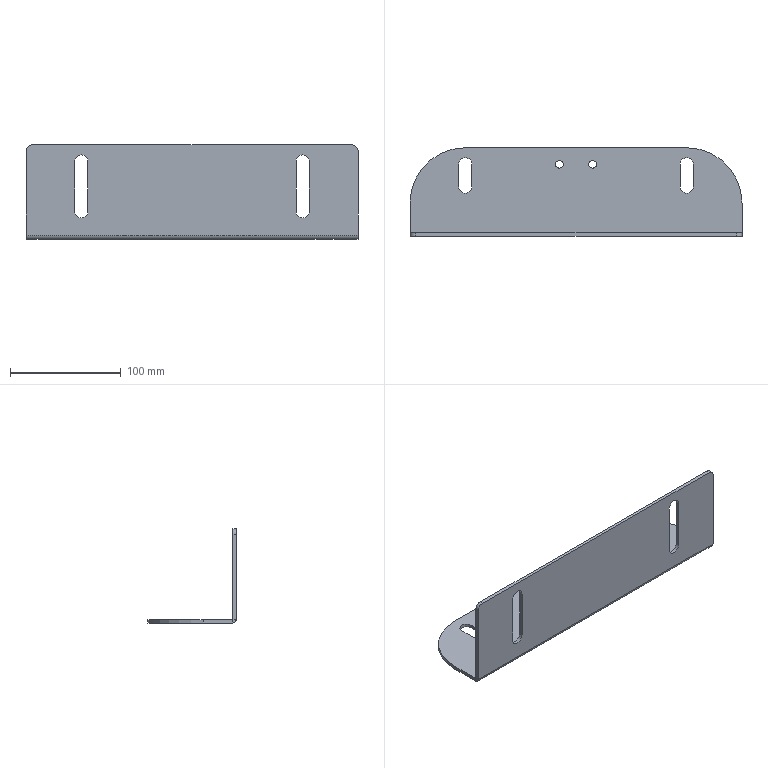Part | SolidWorks | features Fillet 2, ICE 2, EdgeFlange 1, FlatPattern 1, HoleWzd 1, SMBaseFlange 1, SheetMetal 1 | 1 solid | 40 faces | box 300 x 80 x 85 mm | volume 135508 mm3 | cylinder 20 | plane 20 | commonest cylinder face diameters 12 x10 7 x5 10 x2 100 x2 1 x1
STEP:
#1=CARTESIAN_POINT('',(-18.5,25.,-3.));
#2=VERTEX_POINT('',#1);
#3=CARTESIAN_POINT('',(-11.5,25.,-3.));
#4=VERTEX_POINT('',#3);
#5=CARTESIAN_POINT('',(-15.,25.,-3.));
#6=DIRECTION('',(0.,0.,1.));
#7=DIRECTION('',(1.,0.,0.));
#8=AXIS2_PLACEMENT_3D('',#5,#6,#7);
#9=CIRCLE('',#8,3.5);
#10=EDGE_CURVE('',#2,#4,#9,.T.);
#11=ORIENTED_EDGE('',*,*,#10,.F.);
#12=CARTESIAN_POINT('',(-18.5,25.,0.));
#13=VERTEX_POINT('',#12);
#14=CARTESIAN_POINT('',(-18.5,25.,0.));
#15=DIRECTION('',(0.,0.,1.));
#16=VECTOR('',#15,1000.);
#17=LINE('',#14,#16);
#18=EDGE_CURVE('',#2,#13,#17,.T.);
#19=ORIENTED_EDGE('',*,*,#18,.T.);
#20=CARTESIAN_POINT('',(-11.5,25.,0.));
#21=VERTEX_POINT('',#20);
#22=CARTESIAN_POINT('',(-15.,25.,0.));
#23=DIRECTION('',(0.,0.,1.));
#24=DIRECTION('',(1.,0.,0.));
#25=AXIS2_PLACEMENT_3D('',#22,#23,#24);
#26=CIRCLE('',#25,3.5);
#27=EDGE_CURVE('',#13,#21,#26,.T.);
#28=ORIENTED_EDGE('',*,*,#27,.T.);
#29=CARTESIAN_POINT('',(-11.5,25.,0.));
#30=DIRECTION('',(0.,0.,1.));
#31=VECTOR('',#30,1000.);
#32=LINE('',#29,#31);
#33=EDGE_CURVE('',#4,#21,#32,.T.);
#34=ORIENTED_EDGE('',*,*,#33,.F.);
#35=EDGE_LOOP('',(#11,#19,#28,#34));
#36=FACE_OUTER_BOUND('',#35,.T.);
#37=CARTESIAN_POINT('',(-15.,25.,0.));
#38=DIRECTION('',(0.,0.,1.));
#39=DIRECTION('',(1.,0.,0.));
#40=AXIS2_PLACEMENT_3D('',#37,#38,#39);
#41=CYLINDRICAL_SURFACE('',#40,3.5);
#42=ADVANCED_FACE('',(#36),#41,.F.);
#43=CARTESIAN_POINT('',(11.5,25.,-3.));
#44=VERTEX_POINT('',#43);
#45=CARTESIAN_POINT('',(18.5,25.,-3.));
#46=VERTEX_POINT('',#45);
#47=CARTESIAN_POINT('',(15.,25.,-3.));
#48=DIRECTION('',(0.,0.,1.));
#49=DIRECTION('',(1.,0.,0.));
#50=AXIS2_PLACEMENT_3D('',#47,#48,#49);
#51=CIRCLE('',#50,3.5);
#52=EDGE_CURVE('',#44,#46,#51,.T.);
#53=ORIENTED_EDGE('',*,*,#52,.F.);
#54=CARTESIAN_POINT('',(11.5,25.,0.));
#55=VERTEX_POINT('',#54);
#56=CARTESIAN_POINT('',(11.5,25.,0.));
#57=DIRECTION('',(0.,0.,1.));
#58=VECTOR('',#57,1000.);
#59=LINE('',#56,#58);
#60=EDGE_CURVE('',#44,#55,#59,.T.);
#61=ORIENTED_EDGE('',*,*,#60,.T.);
#62=CARTESIAN_POINT('',(18.5,25.,0.));
#63=VERTEX_POINT('',#62);
#64=CARTESIAN_POINT('',(15.,25.,0.));
#65=DIRECTION('',(0.,0.,1.));
#66=DIRECTION('',(1.,0.,0.));
#67=AXIS2_PLACEMENT_3D('',#64,#65,#66);
#68=CIRCLE('',#67,3.5);
#69=EDGE_CURVE('',#55,#63,#68,.T.);
#70=ORIENTED_EDGE('',*,*,#69,.T.);
#71=CARTESIAN_POINT('',(18.5,25.,0.));
#72=DIRECTION('',(0.,0.,1.));
#73=VECTOR('',#72,1000.);
#74=LINE('',#71,#73);
#75=EDGE_CURVE('',#46,#63,#74,.T.);
#76=ORIENTED_EDGE('',*,*,#75,.F.);
#77=EDGE_LOOP('',(#53,#61,#70,#76));
#78=FACE_OUTER_BOUND('',#77,.T.);
#79=CARTESIAN_POINT('',(15.,25.,0.));
#80=DIRECTION('',(0.,0.,1.));
#81=DIRECTION('',(1.,0.,0.));
#82=AXIS2_PLACEMENT_3D('',#79,#80,#81);
#83=CYLINDRICAL_SURFACE('',#82,3.5);
#84=ADVANCED_FACE('',(#78),#83,.F.);
#85=CARTESIAN_POINT('',(-100.,-40.,73.));
#86=VERTEX_POINT('',#85);
#87=CARTESIAN_POINT('',(-94.,-40.,67.));
#88=VERTEX_POINT('',#87);
#89=CARTESIAN_POINT('',(-100.,-40.,67.));
#90=DIRECTION('',(0.,1.,0.));
#91=DIRECTION('',(0.,0.,1.));
#92=AXIS2_PLACEMENT_3D('',#89,#90,#91);
#93=CIRCLE('',#92,6.);
#94=EDGE_CURVE('',#86,#88,#93,.T.);
#95=ORIENTED_EDGE('',*,*,#94,.F.);
#96=CARTESIAN_POINT('',(-100.,-37.,73.));
#97=VERTEX_POINT('',#96);
#98=CARTESIAN_POINT('',(-100.,-47.,73.));
#99=DIRECTION('',(0.,1.,0.));
#100=VECTOR('',#99,1000.);
#101=LINE('',#98,#100);
#102=EDGE_CURVE('',#86,#97,#101,.T.);
#103=ORIENTED_EDGE('',*,*,#102,.T.);
#104=CARTESIAN_POINT('',(-94.,-37.,67.));
#105=VERTEX_POINT('',#104);
#106=CARTESIAN_POINT('',(-100.,-37.,67.));
#107=DIRECTION('',(0.,1.,0.));
#108=DIRECTION('',(0.,0.,1.));
#109=AXIS2_PLACEMENT_3D('',#106,#107,#108);
#110=CIRCLE('',#109,6.);
#111=EDGE_CURVE('',#97,#105,#110,.T.);
#112=ORIENTED_EDGE('',*,*,#111,.T.);
#113=CARTESIAN_POINT('',(-94.,-47.,67.));
#114=DIRECTION('',(0.,1.,0.));
#115=VECTOR('',#114,1000.);
#116=LINE('',#113,#115);
#117=EDGE_CURVE('',#88,#105,#116,.T.);
#118=ORIENTED_EDGE('',*,*,#117,.F.);
#119=EDGE_LOOP('',(#95,#103,#112,#118));
#120=FACE_OUTER_BOUND('',#119,.T.);
#121=CARTESIAN_POINT('',(-100.,-47.,67.));
#122=DIRECTION('',(0.,1.,0.));
#123=DIRECTION('',(0.,0.,1.));
#124=AXIS2_PLACEMENT_3D('',#121,#122,#123);
#125=CYLINDRICAL_SURFACE('',#124,6.);
#126=ADVANCED_FACE('',(#120),#125,.F.);
#127=CARTESIAN_POINT('',(100.,-40.,73.));
#128=VERTEX_POINT('',#127);
#129=CARTESIAN_POINT('',(106.,-40.,67.));
#130=VERTEX_POINT('',#129);
#131=CARTESIAN_POINT('',(100.,-40.,67.));
#132=DIRECTION('',(0.,1.,0.));
#133=DIRECTION('',(0.,0.,1.));
#134=AXIS2_PLACEMENT_3D('',#131,#132,#133);
#135=CIRCLE('',#134,6.);
#136=EDGE_CURVE('',#128,#130,#135,.T.);
#137=ORIENTED_EDGE('',*,*,#136,.F.);
#138=CARTESIAN_POINT('',(100.,-37.,73.));
#139=VERTEX_POINT('',#138);
#140=CARTESIAN_POINT('',(100.,-47.,73.));
#141=DIRECTION('',(0.,1.,0.));
#142=VECTOR('',#141,1000.);
#143=LINE('',#140,#142);
#144=EDGE_CURVE('',#128,#139,#143,.T.);
#145=ORIENTED_EDGE('',*,*,#144,.T.);
#146=CARTESIAN_POINT('',(106.,-37.,67.));
#147=VERTEX_POINT('',#146);
#148=CARTESIAN_POINT('',(100.,-37.,67.));
#149=DIRECTION('',(0.,1.,0.));
#150=DIRECTION('',(0.,0.,-1.));
#151=AXIS2_PLACEMENT_3D('',#148,#149,#150);
#152=CIRCLE('',#151,6.);
#153=EDGE_CURVE('',#139,#147,#152,.T.);
#154=ORIENTED_EDGE('',*,*,#153,.T.);
#155=CARTESIAN_POINT('',(106.,-47.,67.));
#156=DIRECTION('',(0.,1.,0.));
#157=VECTOR('',#156,1000.);
#158=LINE('',#155,#157);
#159=EDGE_CURVE('',#130,#147,#158,.T.);
#160=ORIENTED_EDGE('',*,*,#159,.F.);
#161=EDGE_LOOP('',(#137,#145,#154,#160));
#162=FACE_OUTER_BOUND('',#161,.T.);
#163=CARTESIAN_POINT('',(100.,-47.,67.));
#164=DIRECTION('',(0.,1.,0.));
#165=DIRECTION('',(0.,0.,1.));
#166=AXIS2_PLACEMENT_3D('',#163,#164,#165);
#167=CYLINDRICAL_SURFACE('',#166,6.);
#168=ADVANCED_FACE('',(#162),#167,.F.);
#169=CARTESIAN_POINT('',(150.,-36.5,-3.));
#170=VERTEX_POINT('',#169);
#171=CARTESIAN_POINT('',(150.,-10.,-3.));
#172=VERTEX_POINT('',#171);
#173=CARTESIAN_POINT('',(150.,40.,-3.));
#174=DIRECTION('',(0.,1.,0.));
#175=VECTOR('',#174,1000.);
#176=LINE('',#173,#175);
#177=EDGE_CURVE('',#170,#172,#176,.T.);
#178=ORIENTED_EDGE('',*,*,#177,.T.);
#179=CARTESIAN_POINT('',(150.,-10.,0.));
#180=VERTEX_POINT('',#179);
#181=CARTESIAN_POINT('',(150.,-10.,-3.));
#182=DIRECTION('',(0.,0.,1.));
#183=VECTOR('',#182,1000.);
#184=LINE('',#181,#183);
#185=EDGE_CURVE('',#172,#180,#184,.T.);
#186=ORIENTED_EDGE('',*,*,#185,.T.);
#187=CARTESIAN_POINT('',(150.,-36.5,0.));
#188=VERTEX_POINT('',#187);
#189=CARTESIAN_POINT('',(150.,40.,0.));
#190=DIRECTION('',(0.,1.,0.));
#191=VECTOR('',#190,1000.);
#192=LINE('',#189,#191);
#193=EDGE_CURVE('',#188,#180,#192,.T.);
#194=ORIENTED_EDGE('',*,*,#193,.F.);
#195=CARTESIAN_POINT('',(150.,-36.5,0.));
#196=DIRECTION('',(0.,0.,-1.));
#197=VECTOR('',#196,1000.);
#198=LINE('',#195,#197);
#199=EDGE_CURVE('',#188,#170,#198,.T.);
#200=ORIENTED_EDGE('',*,*,#199,.T.);
#201=EDGE_LOOP('',(#178,#186,#194,#200));
#202=FACE_OUTER_BOUND('',#201,.T.);
#203=CARTESIAN_POINT('',(150.,40.,-3.));
#204=DIRECTION('',(1.,0.,0.));
#205=DIRECTION('',(0.,0.,-1.));
#206=AXIS2_PLACEMENT_3D('',#203,#204,#205);
#207=PLANE('',#206);
#208=ADVANCED_FACE('',(#202),#207,.T.);
#209=CARTESIAN_POINT('',(-15.,25.,-3.));
#210=DIRECTION('',(0.,0.,1.));
#211=DIRECTION('',(1.,0.,0.));
#212=AXIS2_PLACEMENT_3D('',#209,#210,#211);
#213=CIRCLE('',#212,3.5);
#214=EDGE_CURVE('',#4,#2,#213,.T.);
#215=ORIENTED_EDGE('',*,*,#214,.T.);
#216=ORIENTED_EDGE('',*,*,#10,.T.);
#217=EDGE_LOOP('',(#215,#216));
#218=FACE_BOUND('',#217,.T.);
#219=CARTESIAN_POINT('',(15.,25.,-3.));
#220=DIRECTION('',(0.,0.,1.));
#221=DIRECTION('',(1.,0.,0.));
#222=AXIS2_PLACEMENT_3D('',#219,#220,#221);
#223=CIRCLE('',#222,3.5);
#224=EDGE_CURVE('',#46,#44,#223,.T.);
#225=ORIENTED_EDGE('',*,*,#224,.T.);
#226=ORIENTED_EDGE('',*,*,#52,.T.);
#227=EDGE_LOOP('',(#225,#226));
#228=FACE_BOUND('',#227,.T.);
#229=CARTESIAN_POINT('',(106.,25.,-3.));
#230=VERTEX_POINT('',#229);
#231=CARTESIAN_POINT('',(106.,5.,-3.));
#232=VERTEX_POINT('',#231);
#233=CARTESIAN_POINT('',(106.,25.,-3.));
#234=DIRECTION('',(0.,-1.,0.));
#235=VECTOR('',#234,1000.);
#236=LINE('',#233,#235);
#237=EDGE_CURVE('',#230,#232,#236,.T.);
#238=ORIENTED_EDGE('',*,*,#237,.F.);
#239=CARTESIAN_POINT('',(94.,25.,-3.));
#240=VERTEX_POINT('',#239);
#241=CARTESIAN_POINT('',(100.,25.,-3.));
#242=DIRECTION('',(0.,0.,-1.));
#243=DIRECTION('',(-1.,0.,0.));
#244=AXIS2_PLACEMENT_3D('',#241,#242,#243);
#245=CIRCLE('',#244,6.);
#246=EDGE_CURVE('',#240,#230,#245,.T.);
#247=ORIENTED_EDGE('',*,*,#246,.F.);
#248=CARTESIAN_POINT('',(94.,5.,-3.));
#249=VERTEX_POINT('',#248);
#250=CARTESIAN_POINT('',(94.,25.,-3.));
#251=DIRECTION('',(0.,1.,0.));
#252=VECTOR('',#251,1000.);
#253=LINE('',#250,#252);
#254=EDGE_CURVE('',#249,#240,#253,.T.);
#255=ORIENTED_EDGE('',*,*,#254,.F.);
#256=CARTESIAN_POINT('',(100.,5.,-3.));
#257=DIRECTION('',(0.,0.,-1.));
#258=DIRECTION('',(-1.,0.,0.));
#259=AXIS2_PLACEMENT_3D('',#256,#257,#258);
#260=CIRCLE('',#259,6.);
#261=EDGE_CURVE('',#232,#249,#260,.T.);
#262=ORIENTED_EDGE('',*,*,#261,.F.);
#263=EDGE_LOOP('',(#238,#247,#255,#262));
#264=FACE_BOUND('',#263,.T.);
#265=CARTESIAN_POINT('',(-94.,25.,-3.));
#266=VERTEX_POINT('',#265);
#267=CARTESIAN_POINT('',(-94.,5.,-3.));
#268=VERTEX_POINT('',#267);
#269=CARTESIAN_POINT('',(-94.,25.,-3.));
#270=DIRECTION('',(0.,-1.,0.));
#271=VECTOR('',#270,1000.);
#272=LINE('',#269,#271);
#273=EDGE_CURVE('',#266,#268,#272,.T.);
#274=ORIENTED_EDGE('',*,*,#273,.F.);
#275=CARTESIAN_POINT('',(-106.,25.,-3.));
#276=VERTEX_POINT('',#275);
#277=CARTESIAN_POINT('',(-100.,25.,-3.));
#278=DIRECTION('',(0.,0.,-1.));
#279=DIRECTION('',(1.,0.,0.));
#280=AXIS2_PLACEMENT_3D('',#277,#278,#279);
#281=CIRCLE('',#280,6.);
#282=EDGE_CURVE('',#276,#266,#281,.T.);
#283=ORIENTED_EDGE('',*,*,#282,.F.);
#284=CARTESIAN_POINT('',(-106.,5.,-3.));
#285=VERTEX_POINT('',#284);
#286=CARTESIAN_POINT('',(-106.,25.,-3.));
#287=DIRECTION('',(0.,1.,0.));
#288=VECTOR('',#287,1000.);
#289=LINE('',#286,#288);
#290=EDGE_CURVE('',#285,#276,#289,.T.);
#291=ORIENTED_EDGE('',*,*,#290,.F.);
#292=CARTESIAN_POINT('',(-100.,5.,-3.));
#293=DIRECTION('',(0.,0.,-1.));
#294=DIRECTION('',(1.,0.,0.));
#295=AXIS2_PLACEMENT_3D('',#292,#293,#294);
#296=CIRCLE('',#295,6.);
#297=EDGE_CURVE('',#268,#285,#296,.T.);
#298=ORIENTED_EDGE('',*,*,#297,.F.);
#299=EDGE_LOOP('',(#274,#283,#291,#298));
#300=FACE_BOUND('',#299,.T.);
#301=CARTESIAN_POINT('',(100.,40.,-3.));
#302=VERTEX_POINT('',#301);
#303=CARTESIAN_POINT('',(-100.,40.,-3.));
#304=VERTEX_POINT('',#303);
#305=CARTESIAN_POINT('',(-150.,40.,-3.));
#306=DIRECTION('',(-1.,0.,0.));
#307=VECTOR('',#306,1000.);
#308=LINE('',#305,#307);
#309=EDGE_CURVE('',#302,#304,#308,.T.);
#310=ORIENTED_EDGE('',*,*,#309,.F.);
#311=CARTESIAN_POINT('',(100.,-10.,-3.));
#312=DIRECTION('',(0.,0.,-1.));
#313=DIRECTION('',(1.,0.,0.));
#314=AXIS2_PLACEMENT_3D('',#311,#312,#313);
#315=CIRCLE('',#314,50.);
#316=EDGE_CURVE('',#302,#172,#315,.T.);
#317=ORIENTED_EDGE('',*,*,#316,.T.);
#318=ORIENTED_EDGE('',*,*,#177,.F.);
#319=CARTESIAN_POINT('',(-150.,-36.5,-3.));
#320=VERTEX_POINT('',#319);
#321=CARTESIAN_POINT('',(150.,-36.5,-3.));
#322=DIRECTION('',(-1.,0.,0.));
#323=VECTOR('',#322,1000.);
#324=LINE('',#321,#323);
#325=EDGE_CURVE('',#170,#320,#324,.T.);
#326=ORIENTED_EDGE('',*,*,#325,.T.);
#327=CARTESIAN_POINT('',(-150.,-10.,-3.));
#328=VERTEX_POINT('',#327);
#329=CARTESIAN_POINT('',(-150.,40.,-3.));
#330=DIRECTION('',(0.,-1.,0.));
#331=VECTOR('',#330,1000.);
#332=LINE('',#329,#331);
#333=EDGE_CURVE('',#328,#320,#332,.T.);
#334=ORIENTED_EDGE('',*,*,#333,.F.);
#335=CARTESIAN_POINT('',(-100.,-10.,-3.));
#336=DIRECTION('',(0.,0.,-1.));
#337=DIRECTION('',(1.,0.,0.));
#338=AXIS2_PLACEMENT_3D('',#335,#336,#337);
#339=CIRCLE('',#338,50.);
#340=EDGE_CURVE('',#328,#304,#339,.T.);
#341=ORIENTED_EDGE('',*,*,#340,.T.);
#342=EDGE_LOOP('',(#310,#317,#318,#326,#334,#341));
#343=FACE_OUTER_BOUND('',#342,.T.);
#344=CARTESIAN_POINT('',(0.,0.,-3.));
#345=DIRECTION('',(0.,0.,1.));
#346=DIRECTION('',(1.,0.,0.));
#347=AXIS2_PLACEMENT_3D('',#344,#345,#346);
#348=PLANE('',#347);
#349=ADVANCED_FACE('',(#218,#228,#264,#300,#343),#348,.F.);
#350=CARTESIAN_POINT('',(-15.,25.,0.));
#351=DIRECTION('',(0.,0.,1.));
#352=DIRECTION('',(1.,0.,0.));
#353=AXIS2_PLACEMENT_3D('',#350,#351,#352);
#354=CIRCLE('',#353,3.5);
#355=EDGE_CURVE('',#21,#13,#354,.T.);
#356=ORIENTED_EDGE('',*,*,#355,.F.);
#357=ORIENTED_EDGE('',*,*,#27,.F.);
#358=EDGE_LOOP('',(#356,#357));
#359=FACE_BOUND('',#358,.T.);
#360=CARTESIAN_POINT('',(15.,25.,0.));
#361=DIRECTION('',(0.,0.,1.));
#362=DIRECTION('',(1.,0.,0.));
#363=AXIS2_PLACEMENT_3D('',#360,#361,#362);
#364=CIRCLE('',#363,3.5);
#365=EDGE_CURVE('',#63,#55,#364,.T.);
#366=ORIENTED_EDGE('',*,*,#365,.F.);
#367=ORIENTED_EDGE('',*,*,#69,.F.);
#368=EDGE_LOOP('',(#366,#367));
#369=FACE_BOUND('',#368,.T.);
#370=CARTESIAN_POINT('',(106.,25.,0.));
#371=VERTEX_POINT('',#370);
#372=CARTESIAN_POINT('',(94.,25.,0.));
#373=VERTEX_POINT('',#372);
#374=CARTESIAN_POINT('',(100.,25.,0.));
#375=DIRECTION('',(0.,0.,1.));
#376=DIRECTION('',(1.,0.,0.));
#377=AXIS2_PLACEMENT_3D('',#374,#375,#376);
#378=CIRCLE('',#377,6.);
#379=EDGE_CURVE('',#371,#373,#378,.T.);
#380=ORIENTED_EDGE('',*,*,#379,.F.);
#381=CARTESIAN_POINT('',(106.,5.,0.));
#382=VERTEX_POINT('',#381);
#383=CARTESIAN_POINT('',(106.,0.,0.));
#384=DIRECTION('',(0.,1.,0.));
#385=VECTOR('',#384,1000.);
#386=LINE('',#383,#385);
#387=EDGE_CURVE('',#382,#371,#386,.T.);
#388=ORIENTED_EDGE('',*,*,#387,.F.);
#389=CARTESIAN_POINT('',(94.,5.,0.));
#390=VERTEX_POINT('',#389);
#391=CARTESIAN_POINT('',(100.,5.,0.));
#392=DIRECTION('',(0.,0.,1.));
#393=DIRECTION('',(1.,0.,0.));
#394=AXIS2_PLACEMENT_3D('',#391,#392,#393);
#395=CIRCLE('',#394,6.);
#396=EDGE_CURVE('',#390,#382,#395,.T.);
#397=ORIENTED_EDGE('',*,*,#396,.F.);
#398=CARTESIAN_POINT('',(94.,0.,0.));
#399=DIRECTION('',(0.,-1.,0.));
#400=VECTOR('',#399,1000.);
#401=LINE('',#398,#400);
#402=EDGE_CURVE('',#373,#390,#401,.T.);
#403=ORIENTED_EDGE('',*,*,#402,.F.);
#404=EDGE_LOOP('',(#380,#388,#397,#403));
#405=FACE_BOUND('',#404,.T.);
#406=CARTESIAN_POINT('',(-94.,25.,0.));
#407=VERTEX_POINT('',#406);
#408=CARTESIAN_POINT('',(-106.,25.,0.));
#409=VERTEX_POINT('',#408);
#410=CARTESIAN_POINT('',(-100.,25.,0.));
#411=DIRECTION('',(0.,0.,1.));
#412=DIRECTION('',(1.,0.,0.));
#413=AXIS2_PLACEMENT_3D('',#410,#411,#412);
#414=CIRCLE('',#413,6.);
#415=EDGE_CURVE('',#407,#409,#414,.T.);
#416=ORIENTED_EDGE('',*,*,#415,.F.);
#417=CARTESIAN_POINT('',(-94.,5.,0.));
#418=VERTEX_POINT('',#417);
#419=CARTESIAN_POINT('',(-94.,0.,0.));
#420=DIRECTION('',(0.,1.,0.));
#421=VECTOR('',#420,1000.);
#422=LINE('',#419,#421);
#423=EDGE_CURVE('',#418,#407,#422,.T.);
#424=ORIENTED_EDGE('',*,*,#423,.F.);
#425=CARTESIAN_POINT('',(-106.,5.,0.));
#426=VERTEX_POINT('',#425);
#427=CARTESIAN_POINT('',(-100.,5.,0.));
#428=DIRECTION('',(0.,0.,1.));
#429=DIRECTION('',(1.,0.,0.));
#430=AXIS2_PLACEMENT_3D('',#427,#428,#429);
#431=CIRCLE('',#430,6.);
#432=EDGE_CURVE('',#426,#418,#431,.T.);
#433=ORIENTED_EDGE('',*,*,#432,.F.);
#434=CARTESIAN_POINT('',(-106.,0.,0.));
#435=DIRECTION('',(0.,-1.,0.));
#436=VECTOR('',#435,1000.);
#437=LINE('',#434,#436);
#438=EDGE_CURVE('',#409,#426,#437,.T.);
#439=ORIENTED_EDGE('',*,*,#438,.F.);
#440=EDGE_LOOP('',(#416,#424,#433,#439));
#441=FACE_BOUND('',#440,.T.);
#442=ORIENTED_EDGE('',*,*,#193,.T.);
#443=CARTESIAN_POINT('',(100.,40.,0.));
#444=VERTEX_POINT('',#443);
#445=CARTESIAN_POINT('',(100.,-10.,0.));
#446=DIRECTION('',(0.,0.,1.));
#447=DIRECTION('',(1.,0.,0.));
#448=AXIS2_PLACEMENT_3D('',#445,#446,#447);
#449=CIRCLE('',#448,50.);
#450=EDGE_CURVE('',#180,#444,#449,.T.);
#451=ORIENTED_EDGE('',*,*,#450,.T.);
#452=CARTESIAN_POINT('',(-100.,40.,0.));
#453=VERTEX_POINT('',#452);
#454=CARTESIAN_POINT('',(-150.,40.,0.));
#455=DIRECTION('',(-1.,0.,0.));
#456=VECTOR('',#455,1000.);
#457=LINE('',#454,#456);
#458=EDGE_CURVE('',#444,#453,#457,.T.);
#459=ORIENTED_EDGE('',*,*,#458,.T.);
#460=CARTESIAN_POINT('',(-150.,-10.,0.));
#461=VERTEX_POINT('',#460);
#462=CARTESIAN_POINT('',(-100.,-10.,0.));
#463=DIRECTION('',(0.,0.,1.));
#464=DIRECTION('',(1.,0.,0.));
#465=AXIS2_PLACEMENT_3D('',#462,#463,#464);
#466=CIRCLE('',#465,50.);
#467=EDGE_CURVE('',#453,#461,#466,.T.);
#468=ORIENTED_EDGE('',*,*,#467,.T.);
#469=CARTESIAN_POINT('',(-150.,-36.5,0.));
#470=VERTEX_POINT('',#469);
#471=CARTESIAN_POINT('',(-150.,40.,0.));
#472=DIRECTION('',(0.,-1.,0.));
#473=VECTOR('',#472,1000.);
#474=LINE('',#471,#473);
#475=EDGE_CURVE('',#461,#470,#474,.T.);
#476=ORIENTED_EDGE('',*,*,#475,.T.);
#477=CARTESIAN_POINT('',(150.,-36.5,0.));
#478=DIRECTION('',(-1.,0.,0.));
#479=VECTOR('',#478,1000.);
#480=LINE('',#477,#479);
#481=EDGE_CURVE('',#188,#470,#480,.T.);
#482=ORIENTED_EDGE('',*,*,#481,.F.);
#483=EDGE_LOOP('',(#442,#451,#459,#468,#476,#482));
#484=FACE_OUTER_BOUND('',#483,.T.);
#485=CARTESIAN_POINT('',(0.,0.,0.));
#486=DIRECTION('',(0.,0.,1.));
#487=DIRECTION('',(1.,0.,0.));
#488=AXIS2_PLACEMENT_3D('',#485,#486,#487);
#489=PLANE('',#488);
#490=ADVANCED_FACE('',(#359,#369,#405,#441,#484),#489,.T.);
#491=ORIENTED_EDGE('',*,*,#475,.F.);
#492=CARTESIAN_POINT('',(-150.,-10.,-3.));
#493=DIRECTION('',(0.,0.,-1.));
#494=VECTOR('',#493,1000.);
#495=LINE('',#492,#494);
#496=EDGE_CURVE('',#461,#328,#495,.T.);
#497=ORIENTED_EDGE('',*,*,#496,.T.);
#498=ORIENTED_EDGE('',*,*,#333,.T.);
#499=CARTESIAN_POINT('',(-150.,-36.5,0.));
#500=DIRECTION('',(0.,0.,-1.));
#501=VECTOR('',#500,1000.);
#502=LINE('',#499,#501);
#503=EDGE_CURVE('',#470,#320,#502,.T.);
#504=ORIENTED_EDGE('',*,*,#503,.F.);
#505=EDGE_LOOP('',(#491,#497,#498,#504));
#506=FACE_OUTER_BOUND('',#505,.T.);
#507=CARTESIAN_POINT('',(-150.,40.,-3.));
#508=DIRECTION('',(-1.,0.,0.));
#509=DIRECTION('',(0.,-1.,0.));
#510=AXIS2_PLACEMENT_3D('',#507,#508,#509);
#511=PLANE('',#510);
#512=ADVANCED_FACE('',(#506),#511,.T.);
#513=ORIENTED_EDGE('',*,*,#458,.F.);
#514=CARTESIAN_POINT('',(100.,40.,-3.));
#515=DIRECTION('',(0.,0.,-1.));
#516=VECTOR('',#515,1000.);
#517=LINE('',#514,#516);
#518=EDGE_CURVE('',#444,#302,#517,.T.);
#519=ORIENTED_EDGE('',*,*,#518,.T.);
#520=ORIENTED_EDGE('',*,*,#309,.T.);
#521=CARTESIAN_POINT('',(-100.,40.,-3.));
#522=DIRECTION('',(0.,0.,1.));
#523=VECTOR('',#522,1000.);
#524=LINE('',#521,#523);
#525=EDGE_CURVE('',#304,#453,#524,.T.);
#526=ORIENTED_EDGE('',*,*,#525,.T.);
#527=EDGE_LOOP('',(#513,#519,#520,#526));
#528=FACE_OUTER_BOUND('',#527,.T.);
#529=CARTESIAN_POINT('',(-150.,40.,-3.));
#530=DIRECTION('',(0.,1.,0.));
#531=DIRECTION('',(0.,0.,1.));
#532=AXIS2_PLACEMENT_3D('',#529,#530,#531);
#533=PLANE('',#532);
#534=ADVANCED_FACE('',(#528),#533,.T.);
#535=CARTESIAN_POINT('',(-150.,-37.,0.5));
#536=VERTEX_POINT('',#535);
#537=CARTESIAN_POINT('',(-150.,-40.,0.5));
#538=VERTEX_POINT('',#537);
#539=CARTESIAN_POINT('',(-150.,-40.,0.5));
#540=DIRECTION('',(0.,-1.,0.));
#541=VECTOR('',#540,1000.);
#542=LINE('',#539,#541);
#543=EDGE_CURVE('',#536,#538,#542,.T.);
#544=ORIENTED_EDGE('',*,*,#543,.F.);
#545=CARTESIAN_POINT('',(-150.,-36.5,0.5));
#546=DIRECTION('',(-1.,0.,0.));
#547=DIRECTION('',(0.,0.,-1.));
#548=AXIS2_PLACEMENT_3D('',#545,#546,#547);
#549=CIRCLE('',#548,0.5);
#550=EDGE_CURVE('',#470,#536,#549,.T.);
#551=ORIENTED_EDGE('',*,*,#550,.F.);
#552=ORIENTED_EDGE('',*,*,#503,.T.);
#553=CARTESIAN_POINT('',(-150.,-36.5,0.5));
#554=DIRECTION('',(-1.,0.,0.));
#555=DIRECTION('',(0.,0.,-1.));
#556=AXIS2_PLACEMENT_3D('',#553,#554,#555);
#557=CIRCLE('',#556,3.5);
#558=EDGE_CURVE('',#320,#538,#557,.T.);
#559=ORIENTED_EDGE('',*,*,#558,.T.);
#560=EDGE_LOOP('',(#544,#551,#552,#559));
#561=FACE_OUTER_BOUND('',#560,.T.);
#562=CARTESIAN_POINT('',(-150.,-36.5,0.5));
#563=DIRECTION('',(-1.,0.,0.));
#564=DIRECTION('',(0.,0.,1.));
#565=AXIS2_PLACEMENT_3D('',#562,#563,#564);
#566=PLANE('',#565);
#567=ADVANCED_FACE('',(#561),#566,.T.);
#568=CARTESIAN_POINT('',(150.,-37.,0.5));
#569=VERTEX_POINT('',#568);
#570=CARTESIAN_POINT('',(150.,-36.5,0.5));
#571=DIRECTION('',(1.,0.,0.));
#572=DIRECTION('',(0.,0.,-1.));
#573=AXIS2_PLACEMENT_3D('',#570,#571,#572);
#574=CIRCLE('',#573,0.5);
#575=EDGE_CURVE('',#569,#188,#574,.T.);
#576=ORIENTED_EDGE('',*,*,#575,.F.);
#577=CARTESIAN_POINT('',(150.,-40.,0.5));
#578=VERTEX_POINT('',#577);
#579=CARTESIAN_POINT('',(150.,-37.,0.5));
#580=DIRECTION('',(0.,-1.,0.));
#581=VECTOR('',#580,1000.);
#582=LINE('',#579,#581);
#583=EDGE_CURVE('',#569,#578,#582,.T.);
#584=ORIENTED_EDGE('',*,*,#583,.T.);
#585=CARTESIAN_POINT('',(150.,-36.5,0.5));
#586=DIRECTION('',(1.,0.,0.));
#587=DIRECTION('',(0.,0.,-1.));
#588=AXIS2_PLACEMENT_3D('',#585,#586,#587);
#589=CIRCLE('',#588,3.5);
#590=EDGE_CURVE('',#578,#170,#589,.T.);
#591=ORIENTED_EDGE('',*,*,#590,.T.);
#592=ORIENTED_EDGE('',*,*,#199,.F.);
#593=EDGE_LOOP('',(#576,#584,#591,#592));
#594=FACE_OUTER_BOUND('',#593,.T.);
#595=CARTESIAN_POINT('',(150.,-36.5,0.5));
#596=DIRECTION('',(-1.,0.,0.));
#597=DIRECTION('',(0.,0.,1.));
#598=AXIS2_PLACEMENT_3D('',#595,#596,#597);
#599=PLANE('',#598);
#600=ADVANCED_FACE('',(#594),#599,.F.);
#601=ORIENTED_EDGE('',*,*,#325,.F.);
#602=ORIENTED_EDGE('',*,*,#590,.F.);
#603=CARTESIAN_POINT('',(-150.,-40.,0.5));
#604=DIRECTION('',(-1.,0.,0.));
#605=VECTOR('',#604,1000.);
#606=LINE('',#603,#605);
#607=EDGE_CURVE('',#578,#538,#606,.T.);
#608=ORIENTED_EDGE('',*,*,#607,.T.);
#609=ORIENTED_EDGE('',*,*,#558,.F.);
#610=EDGE_LOOP('',(#601,#602,#608,#609));
#611=FACE_OUTER_BOUND('',#610,.T.);
#612=CARTESIAN_POINT('',(150.,-36.5,0.5));
#613=DIRECTION('',(1.,0.,0.));
#614=DIRECTION('',(0.,-1.,0.));
#615=AXIS2_PLACEMENT_3D('',#612,#613,#614);
#616=CYLINDRICAL_SURFACE('',#615,3.5);
#617=ADVANCED_FACE('',(#611),#616,.T.);
#618=ORIENTED_EDGE('',*,*,#481,.T.);
#619=ORIENTED_EDGE('',*,*,#550,.T.);
#620=CARTESIAN_POINT('',(-150.,-37.,0.5));
#621=DIRECTION('',(1.,0.,0.));
#622=VECTOR('',#621,1000.);
#623=LINE('',#620,#622);
#624=EDGE_CURVE('',#536,#569,#623,.T.);
#625=ORIENTED_EDGE('',*,*,#624,.T.);
#626=ORIENTED_EDGE('',*,*,#575,.T.);
#627=EDGE_LOOP('',(#618,#619,#625,#626));
#628=FACE_OUTER_BOUND('',#627,.T.);
#629=CARTESIAN_POINT('',(150.,-36.5,0.5));
#630=DIRECTION('',(1.,0.,0.));
#631=DIRECTION('',(0.,-1.,0.));
#632=AXIS2_PLACEMENT_3D('',#629,#630,#631);
#633=CYLINDRICAL_SURFACE('',#632,0.5);
#634=ADVANCED_FACE('',(#628),#633,.F.);
#635=CARTESIAN_POINT('',(-150.,-40.,77.));
#636=VERTEX_POINT('',#635);
#637=CARTESIAN_POINT('',(-150.,-40.,0.));
#638=DIRECTION('',(0.,0.,-1.));
#639=VECTOR('',#638,1000.);
#640=LINE('',#637,#639);
#641=EDGE_CURVE('',#636,#538,#640,.T.);
#642=ORIENTED_EDGE('',*,*,#641,.F.);
#643=CARTESIAN_POINT('',(-150.,-37.,77.));
#644=VERTEX_POINT('',#643);
#645=CARTESIAN_POINT('',(-150.,-40.,77.));
#646=DIRECTION('',(0.,1.,0.));
#647=VECTOR('',#646,1000.);
#648=LINE('',#645,#647);
#649=EDGE_CURVE('',#636,#644,#648,.T.);
#650=ORIENTED_EDGE('',*,*,#649,.T.);
#651=CARTESIAN_POINT('',(-150.,-37.,0.));
#652=DIRECTION('',(0.,0.,-1.));
#653=VECTOR('',#652,1000.);
#654=LINE('',#651,#653);
#655=EDGE_CURVE('',#644,#536,#654,.T.);
#656=ORIENTED_EDGE('',*,*,#655,.T.);
#657=ORIENTED_EDGE('',*,*,#543,.T.);
#658=EDGE_LOOP('',(#642,#650,#656,#657));
#659=FACE_OUTER_BOUND('',#658,.T.);
#660=CARTESIAN_POINT('',(-150.,-40.,0.));
#661=DIRECTION('',(1.,0.,0.));
#662=DIRECTION('',(0.,0.,-1.));
#663=AXIS2_PLACEMENT_3D('',#660,#661,#662);
#664=PLANE('',#663);
#665=ADVANCED_FACE('',(#659),#664,.F.);
#666=CARTESIAN_POINT('',(150.,-37.,77.));
#667=VERTEX_POINT('',#666);
#668=CARTESIAN_POINT('',(150.,-37.,82.));
#669=DIRECTION('',(0.,0.,1.));
#670=VECTOR('',#669,1000.);
#671=LINE('',#668,#670);
#672=EDGE_CURVE('',#569,#667,#671,.T.);
#673=ORIENTED_EDGE('',*,*,#672,.T.);
#674=CARTESIAN_POINT('',(150.,-40.,77.));
#675=VERTEX_POINT('',#674);
#676=CARTESIAN_POINT('',(150.,-40.,77.));
#677=DIRECTION('',(0.,-1.,0.));
#678=VECTOR('',#677,1000.);
#679=LINE('',#676,#678);
#680=EDGE_CURVE('',#667,#675,#679,.T.);
#681=ORIENTED_EDGE('',*,*,#680,.T.);
#682=CARTESIAN_POINT('',(150.,-40.,0.));
#683=DIRECTION('',(0.,0.,1.));
#684=VECTOR('',#683,1000.);
#685=LINE('',#682,#684);
#686=EDGE_CURVE('',#578,#675,#685,.T.);
#687=ORIENTED_EDGE('',*,*,#686,.F.);
#688=ORIENTED_EDGE('',*,*,#583,.F.);
#689=EDGE_LOOP('',(#673,#681,#687,#688));
#690=FACE_OUTER_BOUND('',#689,.T.);
#691=CARTESIAN_POINT('',(150.,-40.,82.));
#692=DIRECTION('',(-1.,0.,0.));
#693=DIRECTION('',(0.,0.,1.));
#694=AXIS2_PLACEMENT_3D('',#691,#692,#693);
#695=PLANE('',#694);
#696=ADVANCED_FACE('',(#690),#695,.F.);
#697=CARTESIAN_POINT('',(-94.,-40.,22.));
#698=VERTEX_POINT('',#697);
#699=CARTESIAN_POINT('',(-94.,-40.,0.));
#700=DIRECTION('',(0.,0.,-1.));
#701=VECTOR('',#700,1000.);
#702=LINE('',#699,#701);
#703=EDGE_CURVE('',#88,#698,#702,.T.);
#704=ORIENTED_EDGE('',*,*,#703,.T.);
#705=CARTESIAN_POINT('',(-106.,-40.,22.));
#706=VERTEX_POINT('',#705);
#707=CARTESIAN_POINT('',(-100.,-40.,22.));
#708=DIRECTION('',(0.,1.,0.));
#709=DIRECTION('',(0.,0.,1.));
#710=AXIS2_PLACEMENT_3D('',#707,#708,#709);
#711=CIRCLE('',#710,6.);
#712=EDGE_CURVE('',#698,#706,#711,.T.);
#713=ORIENTED_EDGE('',*,*,#712,.T.);
#714=CARTESIAN_POINT('',(-106.,-40.,67.));
#715=VERTEX_POINT('',#714);
#716=CARTESIAN_POINT('',(-106.,-40.,0.));
#717=DIRECTION('',(0.,0.,1.));
#718=VECTOR('',#717,1000.);
#719=LINE('',#716,#718);
#720=EDGE_CURVE('',#706,#715,#719,.T.);
#721=ORIENTED_EDGE('',*,*,#720,.T.);
#722=CARTESIAN_POINT('',(-100.,-40.,67.));
#723=DIRECTION('',(0.,1.,0.));
#724=DIRECTION('',(0.,0.,1.));
#725=AXIS2_PLACEMENT_3D('',#722,#723,#724);
#726=CIRCLE('',#725,6.);
#727=EDGE_CURVE('',#715,#86,#726,.T.);
#728=ORIENTED_EDGE('',*,*,#727,.T.);
#729=ORIENTED_EDGE('',*,*,#94,.T.);
#730=EDGE_LOOP('',(#704,#713,#721,#728,#729));
#731=FACE_BOUND('',#730,.T.);
#732=CARTESIAN_POINT('',(106.,-40.,22.));
#733=VERTEX_POINT('',#732);
#734=CARTESIAN_POINT('',(106.,-40.,0.));
#735=DIRECTION('',(0.,0.,-1.));
#736=VECTOR('',#735,1000.);
#737=LINE('',#734,#736);
#738=EDGE_CURVE('',#130,#733,#737,.T.);
#739=ORIENTED_EDGE('',*,*,#738,.T.);
#740=CARTESIAN_POINT('',(94.,-40.,22.));
#741=VERTEX_POINT('',#740);
#742=CARTESIAN_POINT('',(100.,-40.,22.));
#743=DIRECTION('',(0.,1.,0.));
#744=DIRECTION('',(0.,0.,1.));
#745=AXIS2_PLACEMENT_3D('',#742,#743,#744);
#746=CIRCLE('',#745,6.);
#747=EDGE_CURVE('',#733,#741,#746,.T.);
#748=ORIENTED_EDGE('',*,*,#747,.T.);
#749=CARTESIAN_POINT('',(94.,-40.,67.));
#750=VERTEX_POINT('',#749);
#751=CARTESIAN_POINT('',(94.,-40.,0.));
#752=DIRECTION('',(0.,0.,1.));
#753=VECTOR('',#752,1000.);
#754=LINE('',#751,#753);
#755=EDGE_CURVE('',#741,#750,#754,.T.);
#756=ORIENTED_EDGE('',*,*,#755,.T.);
#757=CARTESIAN_POINT('',(100.,-40.,67.));
#758=DIRECTION('',(0.,1.,0.));
#759=DIRECTION('',(0.,0.,1.));
#760=AXIS2_PLACEMENT_3D('',#757,#758,#759);
#761=CIRCLE('',#760,6.);
#762=EDGE_CURVE('',#750,#128,#761,.T.);
#763=ORIENTED_EDGE('',*,*,#762,.T.);
#764=ORIENTED_EDGE('',*,*,#136,.T.);
#765=EDGE_LOOP('',(#739,#748,#756,#763,#764));
#766=FACE_BOUND('',#765,.T.);
#767=ORIENTED_EDGE('',*,*,#686,.T.);
#768=CARTESIAN_POINT('',(145.,-40.,82.));
#769=VERTEX_POINT('',#768);
#770=CARTESIAN_POINT('',(145.,-40.,77.));
#771=DIRECTION('',(0.,-1.,0.));
#772=DIRECTION('',(0.,0.,1.));
#773=AXIS2_PLACEMENT_3D('',#770,#771,#772);
#774=CIRCLE('',#773,5.);
#775=EDGE_CURVE('',#675,#769,#774,.T.);
#776=ORIENTED_EDGE('',*,*,#775,.T.);
#777=CARTESIAN_POINT('',(-145.,-40.,82.));
#778=VERTEX_POINT('',#777);
#779=CARTESIAN_POINT('',(0.,-40.,82.));
#780=DIRECTION('',(-1.,0.,0.));
#781=VECTOR('',#780,1000.);
#782=LINE('',#779,#781);
#783=EDGE_CURVE('',#769,#778,#782,.T.);
#784=ORIENTED_EDGE('',*,*,#783,.T.);
#785=CARTESIAN_POINT('',(-145.,-40.,77.));
#786=DIRECTION('',(0.,-1.,0.));
#787=DIRECTION('',(0.,0.,1.));
#788=AXIS2_PLACEMENT_3D('',#785,#786,#787);
#789=CIRCLE('',#788,5.);
#790=EDGE_CURVE('',#778,#636,#789,.T.);
#791=ORIENTED_EDGE('',*,*,#790,.T.);
#792=ORIENTED_EDGE('',*,*,#641,.T.);
#793=ORIENTED_EDGE('',*,*,#607,.F.);
#794=EDGE_LOOP('',(#767,#776,#784,#791,#792,#793));
#795=FACE_OUTER_BOUND('',#794,.T.);
#796=CARTESIAN_POINT('',(0.,-40.,0.));
#797=DIRECTION('',(0.,1.,0.));
#798=DIRECTION('',(0.,0.,1.));
#799=AXIS2_PLACEMENT_3D('',#796,#797,#798);
#800=PLANE('',#799);
#801=ADVANCED_FACE('',(#731,#766,#795),#800,.F.);
#802=CARTESIAN_POINT('',(-94.,-37.,22.));
#803=VERTEX_POINT('',#802);
#804=CARTESIAN_POINT('',(-106.,-37.,22.));
#805=VERTEX_POINT('',#804);
#806=CARTESIAN_POINT('',(-100.,-37.,22.));
#807=DIRECTION('',(0.,1.,0.));
#808=DIRECTION('',(0.,0.,1.));
#809=AXIS2_PLACEMENT_3D('',#806,#807,#808);
#810=CIRCLE('',#809,6.);
#811=EDGE_CURVE('',#803,#805,#810,.T.);
#812=ORIENTED_EDGE('',*,*,#811,.F.);
#813=CARTESIAN_POINT('',(-94.,-37.,22.));
#814=DIRECTION('',(0.,0.,-1.));
#815=VECTOR('',#814,1000.);
#816=LINE('',#813,#815);
#817=EDGE_CURVE('',#105,#803,#816,.T.);
#818=ORIENTED_EDGE('',*,*,#817,.F.);
#819=ORIENTED_EDGE('',*,*,#111,.F.);
#820=CARTESIAN_POINT('',(-106.,-37.,67.));
#821=VERTEX_POINT('',#820);
#822=CARTESIAN_POINT('',(-100.,-37.,67.));
#823=DIRECTION('',(0.,1.,0.));
#824=DIRECTION('',(0.,0.,1.));
#825=AXIS2_PLACEMENT_3D('',#822,#823,#824);
#826=CIRCLE('',#825,6.);
#827=EDGE_CURVE('',#821,#97,#826,.T.);
#828=ORIENTED_EDGE('',*,*,#827,.F.);
#829=CARTESIAN_POINT('',(-106.,-37.,22.));
#830=DIRECTION('',(0.,0.,1.));
#831=VECTOR('',#830,1000.);
#832=LINE('',#829,#831);
#833=EDGE_CURVE('',#805,#821,#832,.T.);
#834=ORIENTED_EDGE('',*,*,#833,.F.);
#835=EDGE_LOOP('',(#812,#818,#819,#828,#834));
#836=FACE_BOUND('',#835,.T.);
#837=CARTESIAN_POINT('',(106.,-37.,22.));
#838=VERTEX_POINT('',#837);
#839=CARTESIAN_POINT('',(94.,-37.,22.));
#840=VERTEX_POINT('',#839);
#841=CARTESIAN_POINT('',(100.,-37.,22.));
#842=DIRECTION('',(0.,1.,0.));
#843=DIRECTION('',(0.,0.,-1.));
#844=AXIS2_PLACEMENT_3D('',#841,#842,#843);
#845=CIRCLE('',#844,6.);
#846=EDGE_CURVE('',#838,#840,#845,.T.);
#847=ORIENTED_EDGE('',*,*,#846,.F.);
#848=CARTESIAN_POINT('',(106.,-37.,22.));
#849=DIRECTION('',(0.,0.,-1.));
#850=VECTOR('',#849,1000.);
#851=LINE('',#848,#850);
#852=EDGE_CURVE('',#147,#838,#851,.T.);
#853=ORIENTED_EDGE('',*,*,#852,.F.);
#854=ORIENTED_EDGE('',*,*,#153,.F.);
#855=CARTESIAN_POINT('',(94.,-37.,67.));
#856=VERTEX_POINT('',#855);
#857=CARTESIAN_POINT('',(100.,-37.,67.));
#858=DIRECTION('',(0.,1.,0.));
#859=DIRECTION('',(0.,0.,-1.));
#860=AXIS2_PLACEMENT_3D('',#857,#858,#859);
#861=CIRCLE('',#860,6.);
#862=EDGE_CURVE('',#856,#139,#861,.T.);
#863=ORIENTED_EDGE('',*,*,#862,.F.);
#864=CARTESIAN_POINT('',(94.,-37.,22.));
#865=DIRECTION('',(0.,0.,1.));
#866=VECTOR('',#865,1000.);
#867=LINE('',#864,#866);
#868=EDGE_CURVE('',#840,#856,#867,.T.);
#869=ORIENTED_EDGE('',*,*,#868,.F.);
#870=EDGE_LOOP('',(#847,#853,#854,#863,#869));
#871=FACE_BOUND('',#870,.T.);
#872=CARTESIAN_POINT('',(145.,-37.,82.));
#873=VERTEX_POINT('',#872);
#874=CARTESIAN_POINT('',(-145.,-37.,82.));
#875=VERTEX_POINT('',#874);
#876=CARTESIAN_POINT('',(-150.,-37.,82.));
#877=DIRECTION('',(-1.,0.,0.));
#878=VECTOR('',#877,1000.);
#879=LINE('',#876,#878);
#880=EDGE_CURVE('',#873,#875,#879,.T.);
#881=ORIENTED_EDGE('',*,*,#880,.F.);
#882=CARTESIAN_POINT('',(145.,-37.,77.));
#883=DIRECTION('',(0.,1.,0.));
#884=DIRECTION('',(0.,0.,1.));
#885=AXIS2_PLACEMENT_3D('',#882,#883,#884);
#886=CIRCLE('',#885,5.);
#887=EDGE_CURVE('',#873,#667,#886,.T.);
#888=ORIENTED_EDGE('',*,*,#887,.T.);
#889=ORIENTED_EDGE('',*,*,#672,.F.);
#890=ORIENTED_EDGE('',*,*,#624,.F.);
#891=ORIENTED_EDGE('',*,*,#655,.F.);
#892=CARTESIAN_POINT('',(-145.,-37.,77.));
#893=DIRECTION('',(0.,1.,0.));
#894=DIRECTION('',(0.,0.,1.));
#895=AXIS2_PLACEMENT_3D('',#892,#893,#894);
#896=CIRCLE('',#895,5.);
#897=EDGE_CURVE('',#644,#875,#896,.T.);
#898=ORIENTED_EDGE('',*,*,#897,.T.);
#899=EDGE_LOOP('',(#881,#888,#889,#890,#891,#898));
#900=FACE_OUTER_BOUND('',#899,.T.);
#901=CARTESIAN_POINT('',(0.,-37.,0.));
#902=DIRECTION('',(0.,1.,0.));
#903=DIRECTION('',(0.,0.,1.));
#904=AXIS2_PLACEMENT_3D('',#901,#902,#903);
#905=PLANE('',#904);
#906=ADVANCED_FACE('',(#836,#871,#900),#905,.T.);
#907=ORIENTED_EDGE('',*,*,#783,.F.);
#908=CARTESIAN_POINT('',(145.,-40.,82.));
#909=DIRECTION('',(0.,1.,0.));
#910=VECTOR('',#909,1000.);
#911=LINE('',#908,#910);
#912=EDGE_CURVE('',#769,#873,#911,.T.);
#913=ORIENTED_EDGE('',*,*,#912,.T.);
#914=ORIENTED_EDGE('',*,*,#880,.T.);
#915=CARTESIAN_POINT('',(-145.,-40.,82.));
#916=DIRECTION('',(0.,-1.,0.));
#917=VECTOR('',#916,1000.);
#918=LINE('',#915,#917);
#919=EDGE_CURVE('',#875,#778,#918,.T.);
#920=ORIENTED_EDGE('',*,*,#919,.T.);
#921=EDGE_LOOP('',(#907,#913,#914,#920));
#922=FACE_OUTER_BOUND('',#921,.T.);
#923=CARTESIAN_POINT('',(-150.,-40.,82.));
#924=DIRECTION('',(0.,0.,-1.));
#925=DIRECTION('',(0.,1.,0.));
#926=AXIS2_PLACEMENT_3D('',#923,#924,#925);
#927=PLANE('',#926);
#928=ADVANCED_FACE('',(#922),#927,.F.);
#929=ORIENTED_EDGE('',*,*,#316,.F.);
#930=ORIENTED_EDGE('',*,*,#518,.F.);
#931=ORIENTED_EDGE('',*,*,#450,.F.);
#932=ORIENTED_EDGE('',*,*,#185,.F.);
#933=EDGE_LOOP('',(#929,#930,#931,#932));
#934=FACE_OUTER_BOUND('',#933,.T.);
#935=CARTESIAN_POINT('',(100.,-10.,-3.));
#936=DIRECTION('',(0.,0.,1.));
#937=DIRECTION('',(1.,0.,0.));
#938=AXIS2_PLACEMENT_3D('',#935,#936,#937);
#939=CYLINDRICAL_SURFACE('',#938,50.);
#940=ADVANCED_FACE('',(#934),#939,.T.);
#941=ORIENTED_EDGE('',*,*,#340,.F.);
#942=ORIENTED_EDGE('',*,*,#496,.F.);
#943=ORIENTED_EDGE('',*,*,#467,.F.);
#944=ORIENTED_EDGE('',*,*,#525,.F.);
#945=EDGE_LOOP('',(#941,#942,#943,#944));
#946=FACE_OUTER_BOUND('',#945,.T.);
#947=CARTESIAN_POINT('',(-100.,-10.,-3.));
#948=DIRECTION('',(0.,0.,1.));
#949=DIRECTION('',(1.,0.,0.));
#950=AXIS2_PLACEMENT_3D('',#947,#948,#949);
#951=CYLINDRICAL_SURFACE('',#950,50.);
#952=ADVANCED_FACE('',(#946),#951,.T.);
#953=ORIENTED_EDGE('',*,*,#415,.T.);
#954=CARTESIAN_POINT('',(-106.,25.,7.));
#955=DIRECTION('',(0.,0.,-1.));
#956=VECTOR('',#955,1000.);
#957=LINE('',#954,#956);
#958=EDGE_CURVE('',#409,#276,#957,.T.);
#959=ORIENTED_EDGE('',*,*,#958,.T.);
#960=ORIENTED_EDGE('',*,*,#282,.T.);
#961=CARTESIAN_POINT('',(-94.,25.,7.));
#962=DIRECTION('',(0.,0.,-1.));
#963=VECTOR('',#962,1000.);
#964=LINE('',#961,#963);
#965=EDGE_CURVE('',#407,#266,#964,.T.);
#966=ORIENTED_EDGE('',*,*,#965,.F.);
#967=EDGE_LOOP('',(#953,#959,#960,#966));
#968=FACE_OUTER_BOUND('',#967,.T.);
#969=CARTESIAN_POINT('',(-100.,25.,7.));
#970=DIRECTION('',(0.,0.,-1.));
#971=DIRECTION('',(-1.,0.,0.));
#972=AXIS2_PLACEMENT_3D('',#969,#970,#971);
#973=CYLINDRICAL_SURFACE('',#972,6.);
#974=ADVANCED_FACE('',(#968),#973,.F.);
#975=ORIENTED_EDGE('',*,*,#438,.T.);
#976=CARTESIAN_POINT('',(-106.,5.,7.));
#977=DIRECTION('',(0.,0.,-1.));
#978=VECTOR('',#977,1000.);
#979=LINE('',#976,#978);
#980=EDGE_CURVE('',#426,#285,#979,.T.);
#981=ORIENTED_EDGE('',*,*,#980,.T.);
#982=ORIENTED_EDGE('',*,*,#290,.T.);
#983=ORIENTED_EDGE('',*,*,#958,.F.);
#984=EDGE_LOOP('',(#975,#981,#982,#983));
#985=FACE_OUTER_BOUND('',#984,.T.);
#986=CARTESIAN_POINT('',(-106.,25.,7.));
#987=DIRECTION('',(-1.,0.,0.));
#988=DIRECTION('',(0.,0.,1.));
#989=AXIS2_PLACEMENT_3D('',#986,#987,#988);
#990=PLANE('',#989);
#991=ADVANCED_FACE('',(#985),#990,.F.);
#992=ORIENTED_EDGE('',*,*,#432,.T.);
#993=CARTESIAN_POINT('',(-94.,5.,7.));
#994=DIRECTION('',(0.,0.,-1.));
#995=VECTOR('',#994,1000.);
#996=LINE('',#993,#995);
#997=EDGE_CURVE('',#418,#268,#996,.T.);
#998=ORIENTED_EDGE('',*,*,#997,.T.);
#999=ORIENTED_EDGE('',*,*,#297,.T.);
#1000=ORIENTED_EDGE('',*,*,#980,.F.);
#1001=EDGE_LOOP('',(#992,#998,#999,#1000));
#1002=FACE_OUTER_BOUND('',#1001,.T.);
#1003=CARTESIAN_POINT('',(-100.,5.,7.));
#1004=DIRECTION('',(0.,0.,-1.));
#1005=DIRECTION('',(-1.,0.,0.));
#1006=AXIS2_PLACEMENT_3D('',#1003,#1004,#1005);
#1007=CYLINDRICAL_SURFACE('',#1006,6.);
#1008=ADVANCED_FACE('',(#1002),#1007,.F.);
#1009=ORIENTED_EDGE('',*,*,#423,.T.);
#1010=ORIENTED_EDGE('',*,*,#965,.T.);
#1011=ORIENTED_EDGE('',*,*,#273,.T.);
#1012=ORIENTED_EDGE('',*,*,#997,.F.);
#1013=EDGE_LOOP('',(#1009,#1010,#1011,#1012));
#1014=FACE_OUTER_BOUND('',#1013,.T.);
#1015=CARTESIAN_POINT('',(-94.,25.,7.));
#1016=DIRECTION('',(1.,0.,0.));
#1017=DIRECTION('',(0.,0.,-1.));
#1018=AXIS2_PLACEMENT_3D('',#1015,#1016,#1017);
#1019=PLANE('',#1018);
#1020=ADVANCED_FACE('',(#1014),#1019,.F.);
#1021=ORIENTED_EDGE('',*,*,#379,.T.);
#1022=CARTESIAN_POINT('',(94.,25.,7.));
#1023=DIRECTION('',(0.,0.,-1.));
#1024=VECTOR('',#1023,1000.);
#1025=LINE('',#1022,#1024);
#1026=EDGE_CURVE('',#373,#240,#1025,.T.);
#1027=ORIENTED_EDGE('',*,*,#1026,.T.);
#1028=ORIENTED_EDGE('',*,*,#246,.T.);
#1029=CARTESIAN_POINT('',(106.,25.,7.));
#1030=DIRECTION('',(0.,0.,-1.));
#1031=VECTOR('',#1030,1000.);
#1032=LINE('',#1029,#1031);
#1033=EDGE_CURVE('',#371,#230,#1032,.T.);
#1034=ORIENTED_EDGE('',*,*,#1033,.F.);
#1035=EDGE_LOOP('',(#1021,#1027,#1028,#1034));
#1036=FACE_OUTER_BOUND('',#1035,.T.);
#1037=CARTESIAN_POINT('',(100.,25.,7.));
#1038=DIRECTION('',(0.,0.,-1.));
#1039=DIRECTION('',(-1.,0.,0.));
#1040=AXIS2_PLACEMENT_3D('',#1037,#1038,#1039);
#1041=CYLINDRICAL_SURFACE('',#1040,6.);
#1042=ADVANCED_FACE('',(#1036),#1041,.F.);
#1043=ORIENTED_EDGE('',*,*,#402,.T.);
#1044=CARTESIAN_POINT('',(94.,5.,7.));
#1045=DIRECTION('',(0.,0.,-1.));
#1046=VECTOR('',#1045,1000.);
#1047=LINE('',#1044,#1046);
#1048=EDGE_CURVE('',#390,#249,#1047,.T.);
#1049=ORIENTED_EDGE('',*,*,#1048,.T.);
#1050=ORIENTED_EDGE('',*,*,#254,.T.);
#1051=ORIENTED_EDGE('',*,*,#1026,.F.);
#1052=EDGE_LOOP('',(#1043,#1049,#1050,#1051));
#1053=FACE_OUTER_BOUND('',#1052,.T.);
#1054=CARTESIAN_POINT('',(94.,25.,7.));
#1055=DIRECTION('',(-1.,0.,0.));
#1056=DIRECTION('',(0.,0.,1.));
#1057=AXIS2_PLACEMENT_3D('',#1054,#1055,#1056);
#1058=PLANE('',#1057);
#1059=ADVANCED_FACE('',(#1053),#1058,.F.);
#1060=ORIENTED_EDGE('',*,*,#396,.T.);
#1061=CARTESIAN_POINT('',(106.,5.,7.));
#1062=DIRECTION('',(0.,0.,-1.));
#1063=VECTOR('',#1062,1000.);
#1064=LINE('',#1061,#1063);
#1065=EDGE_CURVE('',#382,#232,#1064,.T.);
#1066=ORIENTED_EDGE('',*,*,#1065,.T.);
#1067=ORIENTED_EDGE('',*,*,#261,.T.);
#1068=ORIENTED_EDGE('',*,*,#1048,.F.);
#1069=EDGE_LOOP('',(#1060,#1066,#1067,#1068));
#1070=FACE_OUTER_BOUND('',#1069,.T.);
#1071=CARTESIAN_POINT('',(100.,5.,7.));
#1072=DIRECTION('',(0.,0.,-1.));
#1073=DIRECTION('',(-1.,0.,0.));
#1074=AXIS2_PLACEMENT_3D('',#1071,#1072,#1073);
#1075=CYLINDRICAL_SURFACE('',#1074,6.);
#1076=ADVANCED_FACE('',(#1070),#1075,.F.);
#1077=ORIENTED_EDGE('',*,*,#387,.T.);
#1078=ORIENTED_EDGE('',*,*,#1033,.T.);
#1079=ORIENTED_EDGE('',*,*,#237,.T.);
#1080=ORIENTED_EDGE('',*,*,#1065,.F.);
#1081=EDGE_LOOP('',(#1077,#1078,#1079,#1080));
#1082=FACE_OUTER_BOUND('',#1081,.T.);
#1083=CARTESIAN_POINT('',(106.,25.,7.));
#1084=DIRECTION('',(1.,0.,0.));
#1085=DIRECTION('',(0.,0.,-1.));
#1086=AXIS2_PLACEMENT_3D('',#1083,#1084,#1085);
#1087=PLANE('',#1086);
#1088=ADVANCED_FACE('',(#1082),#1087,.F.);
#1089=CARTESIAN_POINT('',(106.,-47.,22.));
#1090=DIRECTION('',(0.,1.,0.));
#1091=VECTOR('',#1090,1000.);
#1092=LINE('',#1089,#1091);
#1093=EDGE_CURVE('',#733,#838,#1092,.T.);
#1094=ORIENTED_EDGE('',*,*,#1093,.T.);
#1095=ORIENTED_EDGE('',*,*,#846,.T.);
#1096=CARTESIAN_POINT('',(94.,-47.,22.));
#1097=DIRECTION('',(0.,1.,0.));
#1098=VECTOR('',#1097,1000.);
#1099=LINE('',#1096,#1098);
#1100=EDGE_CURVE('',#741,#840,#1099,.T.);
#1101=ORIENTED_EDGE('',*,*,#1100,.F.);
#1102=ORIENTED_EDGE('',*,*,#747,.F.);
#1103=EDGE_LOOP('',(#1094,#1095,#1101,#1102));
#1104=FACE_OUTER_BOUND('',#1103,.T.);
#1105=CARTESIAN_POINT('',(100.,-47.,22.));
#1106=DIRECTION('',(0.,1.,0.));
#1107=DIRECTION('',(0.,0.,1.));
#1108=AXIS2_PLACEMENT_3D('',#1105,#1106,#1107);
#1109=CYLINDRICAL_SURFACE('',#1108,6.);
#1110=ADVANCED_FACE('',(#1104),#1109,.F.);
#1111=ORIENTED_EDGE('',*,*,#159,.T.);
#1112=ORIENTED_EDGE('',*,*,#852,.T.);
#1113=ORIENTED_EDGE('',*,*,#1093,.F.);
#1114=ORIENTED_EDGE('',*,*,#738,.F.);
#1115=EDGE_LOOP('',(#1111,#1112,#1113,#1114));
#1116=FACE_OUTER_BOUND('',#1115,.T.);
#1117=CARTESIAN_POINT('',(106.,-47.,22.));
#1118=DIRECTION('',(1.,0.,0.));
#1119=DIRECTION('',(0.,0.,-1.));
#1120=AXIS2_PLACEMENT_3D('',#1117,#1118,#1119);
#1121=PLANE('',#1120);
#1122=ADVANCED_FACE('',(#1116),#1121,.F.);
#1123=ORIENTED_EDGE('',*,*,#144,.F.);
#1124=ORIENTED_EDGE('',*,*,#762,.F.);
#1125=CARTESIAN_POINT('',(94.,-47.,67.));
#1126=DIRECTION('',(0.,1.,0.));
#1127=VECTOR('',#1126,1000.);
#1128=LINE('',#1125,#1127);
#1129=EDGE_CURVE('',#750,#856,#1128,.T.);
#1130=ORIENTED_EDGE('',*,*,#1129,.T.);
#1131=ORIENTED_EDGE('',*,*,#862,.T.);
#1132=EDGE_LOOP('',(#1123,#1124,#1130,#1131));
#1133=FACE_OUTER_BOUND('',#1132,.T.);
#1134=CARTESIAN_POINT('',(100.,-47.,67.));
#1135=DIRECTION('',(0.,1.,0.));
#1136=DIRECTION('',(0.,0.,1.));
#1137=AXIS2_PLACEMENT_3D('',#1134,#1135,#1136);
#1138=CYLINDRICAL_SURFACE('',#1137,6.);
#1139=ADVANCED_FACE('',(#1133),#1138,.F.);
#1140=ORIENTED_EDGE('',*,*,#1100,.T.);
#1141=ORIENTED_EDGE('',*,*,#868,.T.);
#1142=ORIENTED_EDGE('',*,*,#1129,.F.);
#1143=ORIENTED_EDGE('',*,*,#755,.F.);
#1144=EDGE_LOOP('',(#1140,#1141,#1142,#1143));
#1145=FACE_OUTER_BOUND('',#1144,.T.);
#1146=CARTESIAN_POINT('',(94.,-47.,22.));
#1147=DIRECTION('',(-1.,0.,0.));
#1148=DIRECTION('',(0.,0.,1.));
#1149=AXIS2_PLACEMENT_3D('',#1146,#1147,#1148);
#1150=PLANE('',#1149);
#1151=ADVANCED_FACE('',(#1145),#1150,.F.);
#1152=CARTESIAN_POINT('',(-94.,-47.,22.));
#1153=DIRECTION('',(0.,1.,0.));
#1154=VECTOR('',#1153,1000.);
#1155=LINE('',#1152,#1154);
#1156=EDGE_CURVE('',#698,#803,#1155,.T.);
#1157=ORIENTED_EDGE('',*,*,#1156,.T.);
#1158=ORIENTED_EDGE('',*,*,#811,.T.);
#1159=CARTESIAN_POINT('',(-106.,-47.,22.));
#1160=DIRECTION('',(0.,1.,0.));
#1161=VECTOR('',#1160,1000.);
#1162=LINE('',#1159,#1161);
#1163=EDGE_CURVE('',#706,#805,#1162,.T.);
#1164=ORIENTED_EDGE('',*,*,#1163,.F.);
#1165=ORIENTED_EDGE('',*,*,#712,.F.);
#1166=EDGE_LOOP('',(#1157,#1158,#1164,#1165));
#1167=FACE_OUTER_BOUND('',#1166,.T.);
#1168=CARTESIAN_POINT('',(-100.,-47.,22.));
#1169=DIRECTION('',(0.,1.,0.));
#1170=DIRECTION('',(0.,0.,1.));
#1171=AXIS2_PLACEMENT_3D('',#1168,#1169,#1170);
#1172=CYLINDRICAL_SURFACE('',#1171,6.);
#1173=ADVANCED_FACE('',(#1167),#1172,.F.);
#1174=ORIENTED_EDGE('',*,*,#117,.T.);
#1175=ORIENTED_EDGE('',*,*,#817,.T.);
#1176=ORIENTED_EDGE('',*,*,#1156,.F.);
#1177=ORIENTED_EDGE('',*,*,#703,.F.);
#1178=EDGE_LOOP('',(#1174,#1175,#1176,#1177));
#1179=FACE_OUTER_BOUND('',#1178,.T.);
#1180=CARTESIAN_POINT('',(-94.,-47.,22.));
#1181=DIRECTION('',(1.,0.,0.));
#1182=DIRECTION('',(0.,0.,-1.));
#1183=AXIS2_PLACEMENT_3D('',#1180,#1181,#1182);
#1184=PLANE('',#1183);
#1185=ADVANCED_FACE('',(#1179),#1184,.F.);
#1186=ORIENTED_EDGE('',*,*,#102,.F.);
#1187=ORIENTED_EDGE('',*,*,#727,.F.);
#1188=CARTESIAN_POINT('',(-106.,-47.,67.));
#1189=DIRECTION('',(0.,1.,0.));
#1190=VECTOR('',#1189,1000.);
#1191=LINE('',#1188,#1190);
#1192=EDGE_CURVE('',#715,#821,#1191,.T.);
#1193=ORIENTED_EDGE('',*,*,#1192,.T.);
#1194=ORIENTED_EDGE('',*,*,#827,.T.);
#1195=EDGE_LOOP('',(#1186,#1187,#1193,#1194));
#1196=FACE_OUTER_BOUND('',#1195,.T.);
#1197=CARTESIAN_POINT('',(-100.,-47.,67.));
#1198=DIRECTION('',(0.,1.,0.));
#1199=DIRECTION('',(0.,0.,1.));
#1200=AXIS2_PLACEMENT_3D('',#1197,#1198,#1199);
#1201=CYLINDRICAL_SURFACE('',#1200,6.);
#1202=ADVANCED_FACE('',(#1196),#1201,.F.);
#1203=ORIENTED_EDGE('',*,*,#1163,.T.);
#1204=ORIENTED_EDGE('',*,*,#833,.T.);
#1205=ORIENTED_EDGE('',*,*,#1192,.F.);
#1206=ORIENTED_EDGE('',*,*,#720,.F.);
#1207=EDGE_LOOP('',(#1203,#1204,#1205,#1206));
#1208=FACE_OUTER_BOUND('',#1207,.T.);
#1209=CARTESIAN_POINT('',(-106.,-47.,22.));
#1210=DIRECTION('',(-1.,0.,0.));
#1211=DIRECTION('',(0.,0.,1.));
#1212=AXIS2_PLACEMENT_3D('',#1209,#1210,#1211);
#1213=PLANE('',#1212);
#1214=ADVANCED_FACE('',(#1208),#1213,.F.);
#1215=ORIENTED_EDGE('',*,*,#775,.F.);
#1216=ORIENTED_EDGE('',*,*,#680,.F.);
#1217=ORIENTED_EDGE('',*,*,#887,.F.);
#1218=ORIENTED_EDGE('',*,*,#912,.F.);
#1219=EDGE_LOOP('',(#1215,#1216,#1217,#1218));
#1220=FACE_OUTER_BOUND('',#1219,.T.);
#1221=CARTESIAN_POINT('',(145.,-40.,77.));
#1222=DIRECTION('',(0.,1.,0.));
#1223=DIRECTION('',(0.,0.,1.));
#1224=AXIS2_PLACEMENT_3D('',#1221,#1222,#1223);
#1225=CYLINDRICAL_SURFACE('',#1224,5.);
#1226=ADVANCED_FACE('',(#1220),#1225,.T.);
#1227=ORIENTED_EDGE('',*,*,#790,.F.);
#1228=ORIENTED_EDGE('',*,*,#919,.F.);
#1229=ORIENTED_EDGE('',*,*,#897,.F.);
#1230=ORIENTED_EDGE('',*,*,#649,.F.);
#1231=EDGE_LOOP('',(#1227,#1228,#1229,#1230));
#1232=FACE_OUTER_BOUND('',#1231,.T.);
#1233=CARTESIAN_POINT('',(-145.,-40.,77.));
#1234=DIRECTION('',(0.,1.,0.));
#1235=DIRECTION('',(0.,0.,1.));
#1236=AXIS2_PLACEMENT_3D('',#1233,#1234,#1235);
#1237=CYLINDRICAL_SURFACE('',#1236,5.);
#1238=ADVANCED_FACE('',(#1232),#1237,.T.);
#1239=ORIENTED_EDGE('',*,*,#60,.F.);
#1240=ORIENTED_EDGE('',*,*,#224,.F.);
#1241=ORIENTED_EDGE('',*,*,#75,.T.);
#1242=ORIENTED_EDGE('',*,*,#365,.T.);
#1243=EDGE_LOOP('',(#1239,#1240,#1241,#1242));
#1244=FACE_OUTER_BOUND('',#1243,.T.);
#1245=CARTESIAN_POINT('',(15.,25.,0.));
#1246=DIRECTION('',(0.,0.,1.));
#1247=DIRECTION('',(1.,0.,0.));
#1248=AXIS2_PLACEMENT_3D('',#1245,#1246,#1247);
#1249=CYLINDRICAL_SURFACE('',#1248,3.5);
#1250=ADVANCED_FACE('',(#1244),#1249,.F.);
#1251=ORIENTED_EDGE('',*,*,#18,.F.);
#1252=ORIENTED_EDGE('',*,*,#214,.F.);
#1253=ORIENTED_EDGE('',*,*,#33,.T.);
#1254=ORIENTED_EDGE('',*,*,#355,.T.);
#1255=EDGE_LOOP('',(#1251,#1252,#1253,#1254));
#1256=FACE_OUTER_BOUND('',#1255,.T.);
#1257=CARTESIAN_POINT('',(-15.,25.,0.));
#1258=DIRECTION('',(0.,0.,1.));
#1259=DIRECTION('',(1.,0.,0.));
#1260=AXIS2_PLACEMENT_3D('',#1257,#1258,#1259);
#1261=CYLINDRICAL_SURFACE('',#1260,3.5);
#1262=ADVANCED_FACE('',(#1256),#1261,.F.);
#1263=CLOSED_SHELL('',(#42,#84,#126,#168,#208,#349,#490,#512,#534,#567,#600,#617,#634,#665,#696,#801,#906,#928,#940,#952,#974,#991,#1008,#1020,#1042,#1059,#1076,#1088,#1110,#1122,#1139,#1151,#1173,#1185,#1202,#1214,#1226,#1238,#1250,#1262));
#1264=MANIFOLD_SOLID_BREP('',#1263);
#1265=CARTESIAN_POINT('',(0.,0.,0.));
#1266=DIRECTION('',(0.,0.,1.));
#1267=DIRECTION('',(1.,0.,0.));
#1268=AXIS2_PLACEMENT_3D('',#1265,#1266,#1267);
#1269=(LENGTH_UNIT()NAMED_UNIT(*)SI_UNIT(.MILLI.,.METRE.));
#1270=UNCERTAINTY_MEASURE_WITH_UNIT(LENGTH_MEASURE(0.00001),#1269,'','');
#1271=(NAMED_UNIT(*)PLANE_ANGLE_UNIT()SI_UNIT($,.RADIAN.));
#1272=(NAMED_UNIT(*)SI_UNIT($,.STERADIAN.)SOLID_ANGLE_UNIT());
#1273=(GEOMETRIC_REPRESENTATION_CONTEXT(3)GLOBAL_UNCERTAINTY_ASSIGNED_CONTEXT((#1270))GLOBAL_UNIT_ASSIGNED_CONTEXT((#1269,#1271,#1272))REPRESENTATION_CONTEXT('',''));
#1274=ADVANCED_BREP_SHAPE_REPRESENTATION('',(#1264,#1268),#1273);